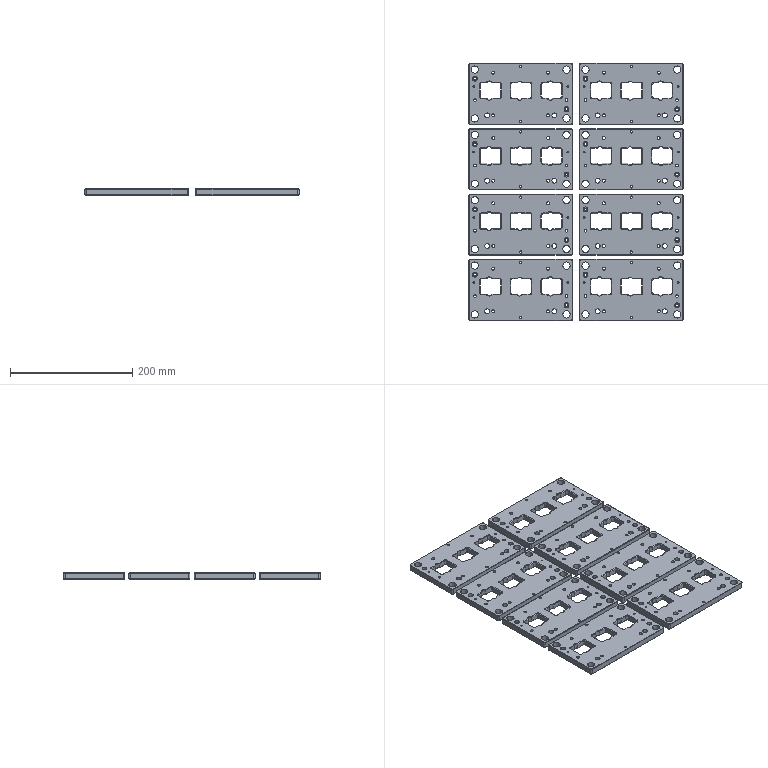Part | 8 solids | 1400 faces | box 351 x 421 x 10 mm | volume 1090075 mm3 | plane 560 | cylinder 496 | cone 344 | commonest cylinder face diameters 3 x64 4.5 x64 4.95 x64 8 x64 12 x64 10 x48